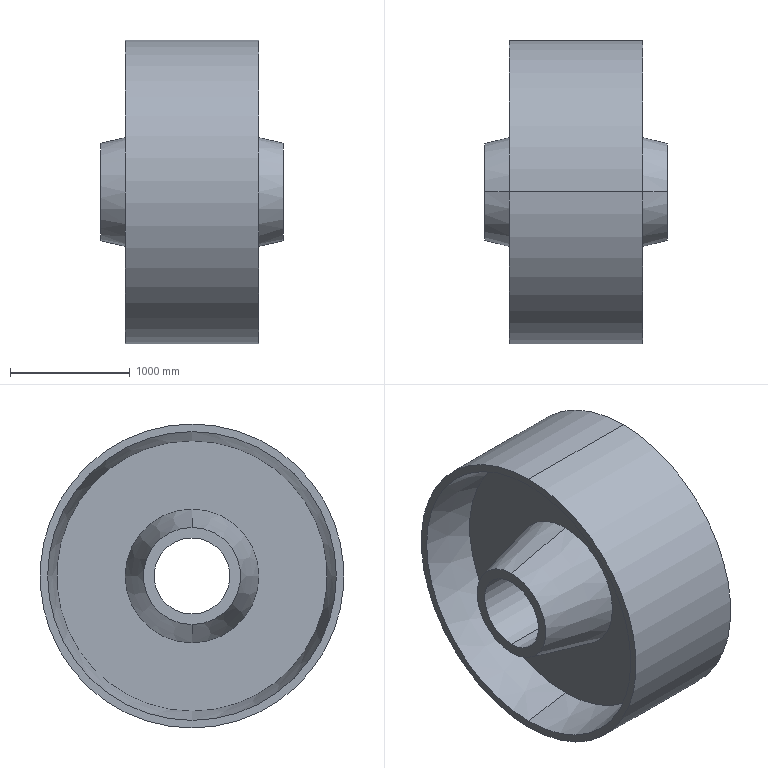Part | SolidWorks | features Revolution 1 | 1 solid | 18 faces | box 1524 x 2540 x 2540 mm | volume 2412190480 mm3 | cone 8 | plane 6 | cylinder 4 | commonest cylinder face diameters 635 x2 2540 x2
STEP:
#1=CARTESIAN_POINT('',(-30.,0.,-16.));
#2=VERTEX_POINT('',#1);
#3=CARTESIAN_POINT('',(-30.,0.,16.));
#4=VERTEX_POINT('',#3);
#5=CARTESIAN_POINT('',(-30.,0.,0.));
#6=DIRECTION('',(1.,0.,0.));
#7=DIRECTION('',(0.,0.,-1.));
#8=AXIS2_PLACEMENT_3D('',#5,#6,#7);
#9=CIRCLE('',#8,16.);
#10=EDGE_CURVE('',#2,#4,#9,.T.);
#11=ORIENTED_EDGE('',*,*,#10,.T.);
#12=CARTESIAN_POINT('',(-5.,0.,22.));
#13=VERTEX_POINT('',#12);
#14=CARTESIAN_POINT('',(-5.,0.,22.));
#15=DIRECTION('',(0.9724,0.,0.2334));
#16=VECTOR('',#15,39.37);
#17=LINE('',#14,#16);
#18=EDGE_CURVE('',#4,#13,#17,.T.);
#19=ORIENTED_EDGE('',*,*,#18,.T.);
#20=CARTESIAN_POINT('',(-5.,0.,-22.));
#21=VERTEX_POINT('',#20);
#22=CARTESIAN_POINT('',(-5.,0.,0.));
#23=DIRECTION('',(1.,0.,0.));
#24=DIRECTION('',(0.,0.,-1.));
#25=AXIS2_PLACEMENT_3D('',#22,#23,#24);
#26=CIRCLE('',#25,22.);
#27=EDGE_CURVE('',#21,#13,#26,.T.);
#28=ORIENTED_EDGE('',*,*,#27,.F.);
#29=CARTESIAN_POINT('',(-5.,0.,-22.));
#30=DIRECTION('',(0.9724,0.,-0.2334));
#31=VECTOR('',#30,39.37);
#32=LINE('',#29,#31);
#33=EDGE_CURVE('',#2,#21,#32,.T.);
#34=ORIENTED_EDGE('',*,*,#33,.F.);
#35=EDGE_LOOP('',(#11,#19,#28,#34));
#36=FACE_OUTER_BOUND('',#35,.T.);
#37=CARTESIAN_POINT('',(-5.,0.,0.));
#38=DIRECTION('',(1.,0.,0.));
#39=DIRECTION('',(0.,0.,-1.));
#40=AXIS2_PLACEMENT_3D('',#37,#38,#39);
#41=CONICAL_SURFACE('',#40,22.,0.2355);
#42=ADVANCED_FACE('',(#36),#41,.T.);
#43=CARTESIAN_POINT('',(-5.,0.,44.5));
#44=VERTEX_POINT('',#43);
#45=CARTESIAN_POINT('',(-5.,0.,-44.5));
#46=VERTEX_POINT('',#45);
#47=CARTESIAN_POINT('',(-5.,0.,0.));
#48=DIRECTION('',(1.,0.,0.));
#49=DIRECTION('',(0.,0.,-1.));
#50=AXIS2_PLACEMENT_3D('',#47,#48,#49);
#51=CIRCLE('',#50,44.5);
#52=EDGE_CURVE('',#44,#46,#51,.T.);
#53=ORIENTED_EDGE('',*,*,#52,.T.);
#54=CARTESIAN_POINT('',(-22.,0.,-47.5));
#55=VERTEX_POINT('',#54);
#56=CARTESIAN_POINT('',(-22.,0.,-47.5));
#57=DIRECTION('',(-0.9848,0.,-0.1738));
#58=VECTOR('',#57,39.37);
#59=LINE('',#56,#58);
#60=EDGE_CURVE('',#46,#55,#59,.T.);
#61=ORIENTED_EDGE('',*,*,#60,.T.);
#62=CARTESIAN_POINT('',(-22.,0.,47.5));
#63=VERTEX_POINT('',#62);
#64=CARTESIAN_POINT('',(-22.,0.,0.));
#65=DIRECTION('',(1.,0.,0.));
#66=DIRECTION('',(0.,0.,-1.));
#67=AXIS2_PLACEMENT_3D('',#64,#65,#66);
#68=CIRCLE('',#67,47.5);
#69=EDGE_CURVE('',#63,#55,#68,.T.);
#70=ORIENTED_EDGE('',*,*,#69,.F.);
#71=CARTESIAN_POINT('',(-22.,0.,47.5));
#72=DIRECTION('',(-0.9848,0.,0.1738));
#73=VECTOR('',#72,39.37);
#74=LINE('',#71,#73);
#75=EDGE_CURVE('',#44,#63,#74,.T.);
#76=ORIENTED_EDGE('',*,*,#75,.F.);
#77=EDGE_LOOP('',(#53,#61,#70,#76));
#78=FACE_OUTER_BOUND('',#77,.T.);
#79=CARTESIAN_POINT('',(-22.,0.,0.));
#80=DIRECTION('',(-1.,0.,0.));
#81=DIRECTION('',(0.,0.,1.));
#82=AXIS2_PLACEMENT_3D('',#79,#80,#81);
#83=CONICAL_SURFACE('',#82,47.5,0.1747);
#84=ADVANCED_FACE('',(#78),#83,.F.);
#85=CARTESIAN_POINT('',(-22.,0.,-50.));
#86=VERTEX_POINT('',#85);
#87=CARTESIAN_POINT('',(-22.,0.,50.));
#88=VERTEX_POINT('',#87);
#89=CARTESIAN_POINT('',(-22.,0.,0.));
#90=DIRECTION('',(1.,0.,0.));
#91=DIRECTION('',(0.,0.,-1.));
#92=AXIS2_PLACEMENT_3D('',#89,#90,#91);
#93=CIRCLE('',#92,50.);
#94=EDGE_CURVE('',#86,#88,#93,.T.);
#95=ORIENTED_EDGE('',*,*,#94,.T.);
#96=CARTESIAN_POINT('',(22.,0.,50.));
#97=VERTEX_POINT('',#96);
#98=CARTESIAN_POINT('',(0.,0.,50.));
#99=DIRECTION('',(1.,0.,0.));
#100=VECTOR('',#99,39.37);
#101=LINE('',#98,#100);
#102=EDGE_CURVE('',#88,#97,#101,.T.);
#103=ORIENTED_EDGE('',*,*,#102,.T.);
#104=CARTESIAN_POINT('',(22.,0.,-50.));
#105=VERTEX_POINT('',#104);
#106=CARTESIAN_POINT('',(22.,0.,0.));
#107=DIRECTION('',(1.,0.,0.));
#108=DIRECTION('',(0.,0.,-1.));
#109=AXIS2_PLACEMENT_3D('',#106,#107,#108);
#110=CIRCLE('',#109,50.);
#111=EDGE_CURVE('',#105,#97,#110,.T.);
#112=ORIENTED_EDGE('',*,*,#111,.F.);
#113=CARTESIAN_POINT('',(0.,0.,-50.));
#114=DIRECTION('',(1.,0.,0.));
#115=VECTOR('',#114,39.37);
#116=LINE('',#113,#115);
#117=EDGE_CURVE('',#86,#105,#116,.T.);
#118=ORIENTED_EDGE('',*,*,#117,.F.);
#119=EDGE_LOOP('',(#95,#103,#112,#118));
#120=FACE_OUTER_BOUND('',#119,.T.);
#121=CARTESIAN_POINT('',(0.,0.,0.));
#122=DIRECTION('',(1.,0.,0.));
#123=DIRECTION('',(0.,0.,-1.));
#124=AXIS2_PLACEMENT_3D('',#121,#122,#123);
#125=CYLINDRICAL_SURFACE('',#124,50.);
#126=ADVANCED_FACE('',(#120),#125,.T.);
#127=CARTESIAN_POINT('',(5.,0.,44.5));
#128=VERTEX_POINT('',#127);
#129=CARTESIAN_POINT('',(5.,0.,-44.5));
#130=VERTEX_POINT('',#129);
#131=CARTESIAN_POINT('',(5.,0.,0.));
#132=DIRECTION('',(1.,0.,0.));
#133=DIRECTION('',(0.,0.,-1.));
#134=AXIS2_PLACEMENT_3D('',#131,#132,#133);
#135=CIRCLE('',#134,44.5);
#136=EDGE_CURVE('',#128,#130,#135,.T.);
#137=ORIENTED_EDGE('',*,*,#136,.F.);
#138=CARTESIAN_POINT('',(22.,0.,47.5));
#139=VERTEX_POINT('',#138);
#140=CARTESIAN_POINT('',(5.,0.,44.5));
#141=DIRECTION('',(0.9848,0.,0.1738));
#142=VECTOR('',#141,39.37);
#143=LINE('',#140,#142);
#144=EDGE_CURVE('',#128,#139,#143,.T.);
#145=ORIENTED_EDGE('',*,*,#144,.T.);
#146=CARTESIAN_POINT('',(22.,0.,-47.5));
#147=VERTEX_POINT('',#146);
#148=CARTESIAN_POINT('',(22.,0.,0.));
#149=DIRECTION('',(1.,0.,0.));
#150=DIRECTION('',(0.,0.,-1.));
#151=AXIS2_PLACEMENT_3D('',#148,#149,#150);
#152=CIRCLE('',#151,47.5);
#153=EDGE_CURVE('',#139,#147,#152,.T.);
#154=ORIENTED_EDGE('',*,*,#153,.T.);
#155=CARTESIAN_POINT('',(5.,0.,-44.5));
#156=DIRECTION('',(0.9848,0.,-0.1738));
#157=VECTOR('',#156,39.37);
#158=LINE('',#155,#157);
#159=EDGE_CURVE('',#130,#147,#158,.T.);
#160=ORIENTED_EDGE('',*,*,#159,.F.);
#161=EDGE_LOOP('',(#137,#145,#154,#160));
#162=FACE_OUTER_BOUND('',#161,.T.);
#163=CARTESIAN_POINT('',(5.,0.,0.));
#164=DIRECTION('',(1.,0.,0.));
#165=DIRECTION('',(0.,0.,-1.));
#166=AXIS2_PLACEMENT_3D('',#163,#164,#165);
#167=CONICAL_SURFACE('',#166,44.5,0.1747);
#168=ADVANCED_FACE('',(#162),#167,.F.);
#169=CARTESIAN_POINT('',(30.,0.,-16.));
#170=VERTEX_POINT('',#169);
#171=CARTESIAN_POINT('',(30.,0.,16.));
#172=VERTEX_POINT('',#171);
#173=CARTESIAN_POINT('',(30.,0.,0.));
#174=DIRECTION('',(1.,0.,0.));
#175=DIRECTION('',(0.,0.,-1.));
#176=AXIS2_PLACEMENT_3D('',#173,#174,#175);
#177=CIRCLE('',#176,16.);
#178=EDGE_CURVE('',#170,#172,#177,.T.);
#179=ORIENTED_EDGE('',*,*,#178,.F.);
#180=CARTESIAN_POINT('',(5.,0.,-22.));
#181=VERTEX_POINT('',#180);
#182=CARTESIAN_POINT('',(30.,0.,-16.));
#183=DIRECTION('',(-0.9724,0.,-0.2334));
#184=VECTOR('',#183,39.37);
#185=LINE('',#182,#184);
#186=EDGE_CURVE('',#170,#181,#185,.T.);
#187=ORIENTED_EDGE('',*,*,#186,.T.);
#188=CARTESIAN_POINT('',(5.,0.,22.));
#189=VERTEX_POINT('',#188);
#190=CARTESIAN_POINT('',(5.,0.,0.));
#191=DIRECTION('',(1.,0.,0.));
#192=DIRECTION('',(0.,0.,-1.));
#193=AXIS2_PLACEMENT_3D('',#190,#191,#192);
#194=CIRCLE('',#193,22.);
#195=EDGE_CURVE('',#181,#189,#194,.T.);
#196=ORIENTED_EDGE('',*,*,#195,.T.);
#197=CARTESIAN_POINT('',(30.,0.,16.));
#198=DIRECTION('',(-0.9724,0.,0.2334));
#199=VECTOR('',#198,39.37);
#200=LINE('',#197,#199);
#201=EDGE_CURVE('',#172,#189,#200,.T.);
#202=ORIENTED_EDGE('',*,*,#201,.F.);
#203=EDGE_LOOP('',(#179,#187,#196,#202));
#204=FACE_OUTER_BOUND('',#203,.T.);
#205=CARTESIAN_POINT('',(30.,0.,0.));
#206=DIRECTION('',(-1.,0.,0.));
#207=DIRECTION('',(0.,0.,1.));
#208=AXIS2_PLACEMENT_3D('',#205,#206,#207);
#209=CONICAL_SURFACE('',#208,16.,0.2355);
#210=ADVANCED_FACE('',(#204),#209,.T.);
#211=CARTESIAN_POINT('',(-30.,0.,12.5));
#212=VERTEX_POINT('',#211);
#213=CARTESIAN_POINT('',(-30.,0.,-12.5));
#214=VERTEX_POINT('',#213);
#215=CARTESIAN_POINT('',(-30.,0.,0.));
#216=DIRECTION('',(1.,0.,0.));
#217=DIRECTION('',(0.,0.,-1.));
#218=AXIS2_PLACEMENT_3D('',#215,#216,#217);
#219=CIRCLE('',#218,12.5);
#220=EDGE_CURVE('',#212,#214,#219,.T.);
#221=ORIENTED_EDGE('',*,*,#220,.F.);
#222=CARTESIAN_POINT('',(30.,0.,12.5));
#223=VERTEX_POINT('',#222);
#224=CARTESIAN_POINT('',(0.,0.,12.5));
#225=DIRECTION('',(1.,0.,0.));
#226=VECTOR('',#225,39.37);
#227=LINE('',#224,#226);
#228=EDGE_CURVE('',#212,#223,#227,.T.);
#229=ORIENTED_EDGE('',*,*,#228,.T.);
#230=CARTESIAN_POINT('',(30.,0.,-12.5));
#231=VERTEX_POINT('',#230);
#232=CARTESIAN_POINT('',(30.,0.,0.));
#233=DIRECTION('',(1.,0.,0.));
#234=DIRECTION('',(0.,0.,-1.));
#235=AXIS2_PLACEMENT_3D('',#232,#233,#234);
#236=CIRCLE('',#235,12.5);
#237=EDGE_CURVE('',#223,#231,#236,.T.);
#238=ORIENTED_EDGE('',*,*,#237,.T.);
#239=CARTESIAN_POINT('',(0.,0.,-12.5));
#240=DIRECTION('',(1.,0.,0.));
#241=VECTOR('',#240,39.37);
#242=LINE('',#239,#241);
#243=EDGE_CURVE('',#214,#231,#242,.T.);
#244=ORIENTED_EDGE('',*,*,#243,.F.);
#245=EDGE_LOOP('',(#221,#229,#238,#244));
#246=FACE_OUTER_BOUND('',#245,.T.);
#247=CARTESIAN_POINT('',(0.,0.,0.));
#248=DIRECTION('',(1.,0.,0.));
#249=DIRECTION('',(0.,0.,-1.));
#250=AXIS2_PLACEMENT_3D('',#247,#248,#249);
#251=CYLINDRICAL_SURFACE('',#250,12.5);
#252=ADVANCED_FACE('',(#246),#251,.F.);
#253=ORIENTED_EDGE('',*,*,#228,.F.);
#254=CARTESIAN_POINT('',(-30.,0.,0.));
#255=DIRECTION('',(1.,0.,0.));
#256=DIRECTION('',(0.,0.,-1.));
#257=AXIS2_PLACEMENT_3D('',#254,#255,#256);
#258=CIRCLE('',#257,12.5);
#259=EDGE_CURVE('',#214,#212,#258,.T.);
#260=ORIENTED_EDGE('',*,*,#259,.F.);
#261=ORIENTED_EDGE('',*,*,#243,.T.);
#262=CARTESIAN_POINT('',(30.,0.,0.));
#263=DIRECTION('',(1.,0.,0.));
#264=DIRECTION('',(0.,0.,-1.));
#265=AXIS2_PLACEMENT_3D('',#262,#263,#264);
#266=CIRCLE('',#265,12.5);
#267=EDGE_CURVE('',#231,#223,#266,.T.);
#268=ORIENTED_EDGE('',*,*,#267,.T.);
#269=EDGE_LOOP('',(#253,#260,#261,#268));
#270=FACE_OUTER_BOUND('',#269,.T.);
#271=CARTESIAN_POINT('',(0.,0.,0.));
#272=DIRECTION('',(1.,0.,0.));
#273=DIRECTION('',(0.,0.,-1.));
#274=AXIS2_PLACEMENT_3D('',#271,#272,#273);
#275=CYLINDRICAL_SURFACE('',#274,12.5);
#276=ADVANCED_FACE('',(#270),#275,.F.);
#277=CARTESIAN_POINT('',(30.,0.,0.));
#278=DIRECTION('',(1.,0.,0.));
#279=DIRECTION('',(0.,0.,-1.));
#280=AXIS2_PLACEMENT_3D('',#277,#278,#279);
#281=CIRCLE('',#280,16.);
#282=EDGE_CURVE('',#172,#170,#281,.T.);
#283=ORIENTED_EDGE('',*,*,#282,.T.);
#284=ORIENTED_EDGE('',*,*,#178,.T.);
#285=EDGE_LOOP('',(#283,#284));
#286=FACE_OUTER_BOUND('',#285,.T.);
#287=ORIENTED_EDGE('',*,*,#267,.F.);
#288=ORIENTED_EDGE('',*,*,#237,.F.);
#289=EDGE_LOOP('',(#287,#288));
#290=FACE_BOUND('',#289,.T.);
#291=CARTESIAN_POINT('',(30.,12.5,0.));
#292=DIRECTION('',(1.,0.,0.));
#293=DIRECTION('',(0.,0.,-1.));
#294=AXIS2_PLACEMENT_3D('',#291,#292,#293);
#295=PLANE('',#294);
#296=ADVANCED_FACE('',(#286,#290),#295,.T.);
#297=ORIENTED_EDGE('',*,*,#186,.F.);
#298=ORIENTED_EDGE('',*,*,#282,.F.);
#299=ORIENTED_EDGE('',*,*,#201,.T.);
#300=CARTESIAN_POINT('',(5.,0.,0.));
#301=DIRECTION('',(1.,0.,0.));
#302=DIRECTION('',(0.,0.,-1.));
#303=AXIS2_PLACEMENT_3D('',#300,#301,#302);
#304=CIRCLE('',#303,22.);
#305=EDGE_CURVE('',#189,#181,#304,.T.);
#306=ORIENTED_EDGE('',*,*,#305,.T.);
#307=EDGE_LOOP('',(#297,#298,#299,#306));
#308=FACE_OUTER_BOUND('',#307,.T.);
#309=CARTESIAN_POINT('',(30.,0.,0.));
#310=DIRECTION('',(-1.,0.,0.));
#311=DIRECTION('',(0.,0.,1.));
#312=AXIS2_PLACEMENT_3D('',#309,#310,#311);
#313=CONICAL_SURFACE('',#312,16.,0.2355);
#314=ADVANCED_FACE('',(#308),#313,.T.);
#315=CARTESIAN_POINT('',(5.,0.,0.));
#316=DIRECTION('',(1.,0.,0.));
#317=DIRECTION('',(0.,0.,-1.));
#318=AXIS2_PLACEMENT_3D('',#315,#316,#317);
#319=CIRCLE('',#318,44.5);
#320=EDGE_CURVE('',#130,#128,#319,.T.);
#321=ORIENTED_EDGE('',*,*,#320,.T.);
#322=ORIENTED_EDGE('',*,*,#136,.T.);
#323=EDGE_LOOP('',(#321,#322));
#324=FACE_OUTER_BOUND('',#323,.T.);
#325=ORIENTED_EDGE('',*,*,#305,.F.);
#326=ORIENTED_EDGE('',*,*,#195,.F.);
#327=EDGE_LOOP('',(#325,#326));
#328=FACE_BOUND('',#327,.T.);
#329=CARTESIAN_POINT('',(5.,22.,0.));
#330=DIRECTION('',(1.,0.,0.));
#331=DIRECTION('',(0.,0.,-1.));
#332=AXIS2_PLACEMENT_3D('',#329,#330,#331);
#333=PLANE('',#332);
#334=ADVANCED_FACE('',(#324,#328),#333,.T.);
#335=ORIENTED_EDGE('',*,*,#144,.F.);
#336=ORIENTED_EDGE('',*,*,#320,.F.);
#337=ORIENTED_EDGE('',*,*,#159,.T.);
#338=CARTESIAN_POINT('',(22.,0.,0.));
#339=DIRECTION('',(1.,0.,0.));
#340=DIRECTION('',(0.,0.,-1.));
#341=AXIS2_PLACEMENT_3D('',#338,#339,#340);
#342=CIRCLE('',#341,47.5);
#343=EDGE_CURVE('',#147,#139,#342,.T.);
#344=ORIENTED_EDGE('',*,*,#343,.T.);
#345=EDGE_LOOP('',(#335,#336,#337,#344));
#346=FACE_OUTER_BOUND('',#345,.T.);
#347=CARTESIAN_POINT('',(5.,0.,0.));
#348=DIRECTION('',(1.,0.,0.));
#349=DIRECTION('',(0.,0.,-1.));
#350=AXIS2_PLACEMENT_3D('',#347,#348,#349);
#351=CONICAL_SURFACE('',#350,44.5,0.1747);
#352=ADVANCED_FACE('',(#346),#351,.F.);
#353=ORIENTED_EDGE('',*,*,#111,.T.);
#354=CARTESIAN_POINT('',(22.,0.,0.));
#355=DIRECTION('',(1.,0.,0.));
#356=DIRECTION('',(0.,0.,-1.));
#357=AXIS2_PLACEMENT_3D('',#354,#355,#356);
#358=CIRCLE('',#357,50.);
#359=EDGE_CURVE('',#97,#105,#358,.T.);
#360=ORIENTED_EDGE('',*,*,#359,.T.);
#361=EDGE_LOOP('',(#353,#360));
#362=FACE_OUTER_BOUND('',#361,.T.);
#363=ORIENTED_EDGE('',*,*,#343,.F.);
#364=ORIENTED_EDGE('',*,*,#153,.F.);
#365=EDGE_LOOP('',(#363,#364));
#366=FACE_BOUND('',#365,.T.);
#367=CARTESIAN_POINT('',(22.,47.5,0.));
#368=DIRECTION('',(1.,0.,0.));
#369=DIRECTION('',(0.,0.,-1.));
#370=AXIS2_PLACEMENT_3D('',#367,#368,#369);
#371=PLANE('',#370);
#372=ADVANCED_FACE('',(#362,#366),#371,.T.);
#373=ORIENTED_EDGE('',*,*,#102,.F.);
#374=CARTESIAN_POINT('',(-22.,0.,0.));
#375=DIRECTION('',(1.,0.,0.));
#376=DIRECTION('',(0.,0.,-1.));
#377=AXIS2_PLACEMENT_3D('',#374,#375,#376);
#378=CIRCLE('',#377,50.);
#379=EDGE_CURVE('',#88,#86,#378,.T.);
#380=ORIENTED_EDGE('',*,*,#379,.T.);
#381=ORIENTED_EDGE('',*,*,#117,.T.);
#382=ORIENTED_EDGE('',*,*,#359,.F.);
#383=EDGE_LOOP('',(#373,#380,#381,#382));
#384=FACE_OUTER_BOUND('',#383,.T.);
#385=CARTESIAN_POINT('',(0.,0.,0.));
#386=DIRECTION('',(1.,0.,0.));
#387=DIRECTION('',(0.,0.,-1.));
#388=AXIS2_PLACEMENT_3D('',#385,#386,#387);
#389=CYLINDRICAL_SURFACE('',#388,50.);
#390=ADVANCED_FACE('',(#384),#389,.T.);
#391=ORIENTED_EDGE('',*,*,#69,.T.);
#392=CARTESIAN_POINT('',(-22.,0.,0.));
#393=DIRECTION('',(1.,0.,0.));
#394=DIRECTION('',(0.,0.,-1.));
#395=AXIS2_PLACEMENT_3D('',#392,#393,#394);
#396=CIRCLE('',#395,47.5);
#397=EDGE_CURVE('',#55,#63,#396,.T.);
#398=ORIENTED_EDGE('',*,*,#397,.T.);
#399=EDGE_LOOP('',(#391,#398));
#400=FACE_BOUND('',#399,.T.);
#401=ORIENTED_EDGE('',*,*,#94,.F.);
#402=ORIENTED_EDGE('',*,*,#379,.F.);
#403=EDGE_LOOP('',(#401,#402));
#404=FACE_OUTER_BOUND('',#403,.T.);
#405=CARTESIAN_POINT('',(-22.,47.5,0.));
#406=DIRECTION('',(-1.,0.,0.));
#407=DIRECTION('',(0.,0.,1.));
#408=AXIS2_PLACEMENT_3D('',#405,#406,#407);
#409=PLANE('',#408);
#410=ADVANCED_FACE('',(#400,#404),#409,.T.);
#411=ORIENTED_EDGE('',*,*,#60,.F.);
#412=CARTESIAN_POINT('',(-5.,0.,0.));
#413=DIRECTION('',(1.,0.,0.));
#414=DIRECTION('',(0.,0.,-1.));
#415=AXIS2_PLACEMENT_3D('',#412,#413,#414);
#416=CIRCLE('',#415,44.5);
#417=EDGE_CURVE('',#46,#44,#416,.T.);
#418=ORIENTED_EDGE('',*,*,#417,.T.);
#419=ORIENTED_EDGE('',*,*,#75,.T.);
#420=ORIENTED_EDGE('',*,*,#397,.F.);
#421=EDGE_LOOP('',(#411,#418,#419,#420));
#422=FACE_OUTER_BOUND('',#421,.T.);
#423=CARTESIAN_POINT('',(-22.,0.,0.));
#424=DIRECTION('',(-1.,0.,0.));
#425=DIRECTION('',(0.,0.,1.));
#426=AXIS2_PLACEMENT_3D('',#423,#424,#425);
#427=CONICAL_SURFACE('',#426,47.5,0.1747);
#428=ADVANCED_FACE('',(#422),#427,.F.);
#429=ORIENTED_EDGE('',*,*,#27,.T.);
#430=CARTESIAN_POINT('',(-5.,0.,0.));
#431=DIRECTION('',(1.,0.,0.));
#432=DIRECTION('',(0.,0.,-1.));
#433=AXIS2_PLACEMENT_3D('',#430,#431,#432);
#434=CIRCLE('',#433,22.);
#435=EDGE_CURVE('',#13,#21,#434,.T.);
#436=ORIENTED_EDGE('',*,*,#435,.T.);
#437=EDGE_LOOP('',(#429,#436));
#438=FACE_BOUND('',#437,.T.);
#439=ORIENTED_EDGE('',*,*,#52,.F.);
#440=ORIENTED_EDGE('',*,*,#417,.F.);
#441=EDGE_LOOP('',(#439,#440));
#442=FACE_OUTER_BOUND('',#441,.T.);
#443=CARTESIAN_POINT('',(-5.,22.,0.));
#444=DIRECTION('',(-1.,0.,0.));
#445=DIRECTION('',(0.,0.,1.));
#446=AXIS2_PLACEMENT_3D('',#443,#444,#445);
#447=PLANE('',#446);
#448=ADVANCED_FACE('',(#438,#442),#447,.T.);
#449=ORIENTED_EDGE('',*,*,#18,.F.);
#450=CARTESIAN_POINT('',(-30.,0.,0.));
#451=DIRECTION('',(1.,0.,0.));
#452=DIRECTION('',(0.,0.,-1.));
#453=AXIS2_PLACEMENT_3D('',#450,#451,#452);
#454=CIRCLE('',#453,16.);
#455=EDGE_CURVE('',#4,#2,#454,.T.);
#456=ORIENTED_EDGE('',*,*,#455,.T.);
#457=ORIENTED_EDGE('',*,*,#33,.T.);
#458=ORIENTED_EDGE('',*,*,#435,.F.);
#459=EDGE_LOOP('',(#449,#456,#457,#458));
#460=FACE_OUTER_BOUND('',#459,.T.);
#461=CARTESIAN_POINT('',(-5.,0.,0.));
#462=DIRECTION('',(1.,0.,0.));
#463=DIRECTION('',(0.,0.,-1.));
#464=AXIS2_PLACEMENT_3D('',#461,#462,#463);
#465=CONICAL_SURFACE('',#464,22.,0.2355);
#466=ADVANCED_FACE('',(#460),#465,.T.);
#467=ORIENTED_EDGE('',*,*,#259,.T.);
#468=ORIENTED_EDGE('',*,*,#220,.T.);
#469=EDGE_LOOP('',(#467,#468));
#470=FACE_BOUND('',#469,.T.);
#471=ORIENTED_EDGE('',*,*,#10,.F.);
#472=ORIENTED_EDGE('',*,*,#455,.F.);
#473=EDGE_LOOP('',(#471,#472));
#474=FACE_OUTER_BOUND('',#473,.T.);
#475=CARTESIAN_POINT('',(-30.,12.5,0.));
#476=DIRECTION('',(-1.,0.,0.));
#477=DIRECTION('',(0.,0.,1.));
#478=AXIS2_PLACEMENT_3D('',#475,#476,#477);
#479=PLANE('',#478);
#480=ADVANCED_FACE('',(#470,#474),#479,.T.);
#481=CLOSED_SHELL('',(#42,#84,#126,#168,#210,#252,#276,#296,#314,#334,#352,#372,#390,#410,#428,#448,#466,#480));
#482=MANIFOLD_SOLID_BREP('',#481);
#483=CARTESIAN_POINT('',(0.,0.,0.));
#484=DIRECTION('',(0.,0.,1.));
#485=DIRECTION('',(1.,0.,0.));
#486=AXIS2_PLACEMENT_3D('',#483,#484,#485);
#487=(LENGTH_UNIT()NAMED_UNIT(*)SI_UNIT($,.METRE.));
#488=LENGTH_MEASURE_WITH_UNIT(LENGTH_MEASURE(0.0254),#487);
#489=DIMENSIONAL_EXPONENTS(1.,0.,0.,0.,0.,0.,0.);
#490=(CONVERSION_BASED_UNIT('INCH',#488)LENGTH_UNIT()NAMED_UNIT(#489));
#491=UNCERTAINTY_MEASURE_WITH_UNIT(LENGTH_MEASURE(0.00001),#490,'','');
#492=(NAMED_UNIT(*)PLANE_ANGLE_UNIT()SI_UNIT($,.RADIAN.));
#493=(NAMED_UNIT(*)SI_UNIT($,.STERADIAN.)SOLID_ANGLE_UNIT());
#494=(GEOMETRIC_REPRESENTATION_CONTEXT(3)GLOBAL_UNCERTAINTY_ASSIGNED_CONTEXT((#491))GLOBAL_UNIT_ASSIGNED_CONTEXT((#490,#492,#493))REPRESENTATION_CONTEXT('',''));
#495=ADVANCED_BREP_SHAPE_REPRESENTATION('',(#482,#486),#494);